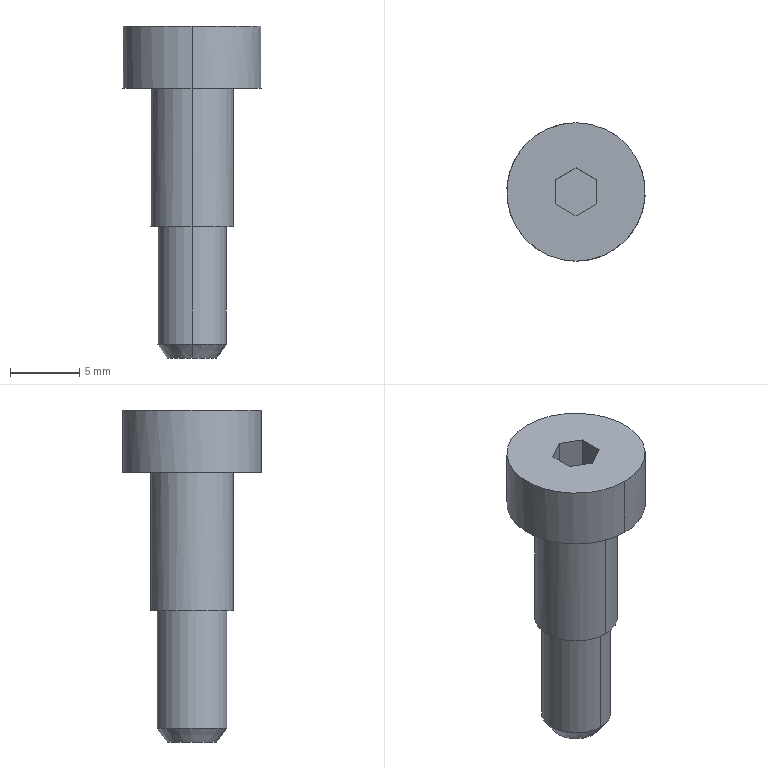Part | CATIA | 1 solid | 19 faces | box 10 x 10 x 24 mm | volume 794.336 mm3 | plane 11 | cylinder 6 | cone 2 | commonest cylinder face diameters 5 x2 6 x2 10 x2
STEP:
#1=CARTESIAN_POINT('',(0.,-2.5,-8.5));
#2=VERTEX_POINT('',#1);
#3=CARTESIAN_POINT('',(0.,-1.8,-9.5));
#4=VERTEX_POINT('',#3);
#5=CARTESIAN_POINT('',(0.,-286789.293,409565.487));
#6=DIRECTION('',(0.,-0.5736,0.8192));
#7=VECTOR('',#6,1.);
#8=LINE('',#5,#7);
#9=EDGE_CURVE('',#2,#4,#8,.F.);
#10=ORIENTED_EDGE('',*,*,#9,.F.);
#11=CARTESIAN_POINT('',(0.,2.5,-8.5));
#12=VERTEX_POINT('',#11);
#13=CARTESIAN_POINT('',(0.,0.,-8.5));
#14=DIRECTION('',(0.,0.,1.));
#15=AXIS2_PLACEMENT_3D('',#13,#14,$);
#16=CIRCLE('',#15,2.5);
#17=EDGE_CURVE('',#2,#12,#16,.F.);
#18=ORIENTED_EDGE('',*,*,#17,.T.);
#19=CARTESIAN_POINT('',(0.,1.8,-9.5));
#20=VERTEX_POINT('',#19);
#21=CARTESIAN_POINT('',(0.,286789.293,409565.487));
#22=DIRECTION('',(0.,0.5736,0.8192));
#23=VECTOR('',#22,1.);
#24=LINE('',#21,#23);
#25=EDGE_CURVE('',#20,#12,#24,.T.);
#26=ORIENTED_EDGE('',*,*,#25,.F.);
#27=CARTESIAN_POINT('',(0.,0.,-9.5));
#28=DIRECTION('',(0.,0.,1.));
#29=AXIS2_PLACEMENT_3D('',#27,#28,$);
#30=CIRCLE('',#29,1.8);
#31=EDGE_CURVE('',#4,#20,#30,.F.);
#32=ORIENTED_EDGE('',*,*,#31,.F.);
#33=EDGE_LOOP('',(#10,#18,#26,#32));
#34=FACE_OUTER_BOUND('',#33,.T.);
#35=CARTESIAN_POINT('',(0.,0.,-9.));
#36=DIRECTION('',(0.,0.,1.));
#37=DIRECTION('',(0.,1.,0.));
#38=AXIS2_PLACEMENT_3D('',#35,#36,#37);
#39=CONICAL_SURFACE('',#38,2.15,0.6109);
#40=ADVANCED_FACE('',(#34),#39,.T.);
#41=ORIENTED_EDGE('',*,*,#9,.T.);
#42=CARTESIAN_POINT('',(0.,0.,-9.5));
#43=DIRECTION('',(0.,0.,1.));
#44=AXIS2_PLACEMENT_3D('',#42,#43,$);
#45=CIRCLE('',#44,1.8);
#46=EDGE_CURVE('',#20,#4,#45,.F.);
#47=ORIENTED_EDGE('',*,*,#46,.F.);
#48=ORIENTED_EDGE('',*,*,#25,.T.);
#49=CARTESIAN_POINT('',(0.,0.,-8.5));
#50=DIRECTION('',(0.,0.,1.));
#51=AXIS2_PLACEMENT_3D('',#49,#50,$);
#52=CIRCLE('',#51,2.5);
#53=EDGE_CURVE('',#12,#2,#52,.F.);
#54=ORIENTED_EDGE('',*,*,#53,.T.);
#55=EDGE_LOOP('',(#41,#47,#48,#54));
#56=FACE_OUTER_BOUND('',#55,.T.);
#57=CARTESIAN_POINT('',(0.,0.,-9.));
#58=DIRECTION('',(0.,0.,1.));
#59=DIRECTION('',(0.,-1.,0.));
#60=AXIS2_PLACEMENT_3D('',#57,#58,#59);
#61=CONICAL_SURFACE('',#60,2.15,0.6109);
#62=ADVANCED_FACE('',(#56),#61,.T.);
#63=CARTESIAN_POINT('',(0.,-2.5,0.));
#64=VERTEX_POINT('',#63);
#65=CARTESIAN_POINT('',(0.,-2.5,-4.25));
#66=DIRECTION('',(0.,0.,1.));
#67=VECTOR('',#66,1.);
#68=LINE('',#65,#67);
#69=EDGE_CURVE('',#64,#2,#68,.F.);
#70=ORIENTED_EDGE('',*,*,#69,.F.);
#71=CARTESIAN_POINT('',(0.,2.5,0.));
#72=VERTEX_POINT('',#71);
#73=CARTESIAN_POINT('',(0.,0.,0.));
#74=DIRECTION('',(0.,0.,1.));
#75=AXIS2_PLACEMENT_3D('',#73,#74,$);
#76=CIRCLE('',#75,2.5);
#77=EDGE_CURVE('',#64,#72,#76,.F.);
#78=ORIENTED_EDGE('',*,*,#77,.T.);
#79=CARTESIAN_POINT('',(0.,2.5,-4.25));
#80=DIRECTION('',(0.,0.,1.));
#81=VECTOR('',#80,1.);
#82=LINE('',#79,#81);
#83=EDGE_CURVE('',#12,#72,#82,.T.);
#84=ORIENTED_EDGE('',*,*,#83,.F.);
#85=ORIENTED_EDGE('',*,*,#17,.F.);
#86=EDGE_LOOP('',(#70,#78,#84,#85));
#87=FACE_OUTER_BOUND('',#86,.T.);
#88=CARTESIAN_POINT('',(0.,0.,-4.25));
#89=DIRECTION('',(0.,0.,1.));
#90=DIRECTION('',(0.,1.,0.));
#91=AXIS2_PLACEMENT_3D('',#88,#89,#90);
#92=CYLINDRICAL_SURFACE('',#91,2.5);
#93=ADVANCED_FACE('',(#87),#92,.T.);
#94=ORIENTED_EDGE('',*,*,#31,.T.);
#95=ORIENTED_EDGE('',*,*,#46,.T.);
#96=EDGE_LOOP('',(#94,#95));
#97=FACE_OUTER_BOUND('',#96,.T.);
#98=CARTESIAN_POINT('',(0.,-0.8999,-9.5));
#99=DIRECTION('',(0.,0.,-1.));
#100=DIRECTION('',(0.,-1.,0.));
#101=AXIS2_PLACEMENT_3D('',#98,#99,#100);
#102=PLANE('',#101);
#103=ADVANCED_FACE('',(#97),#102,.T.);
#104=ORIENTED_EDGE('',*,*,#69,.T.);
#105=ORIENTED_EDGE('',*,*,#53,.F.);
#106=ORIENTED_EDGE('',*,*,#83,.T.);
#107=CARTESIAN_POINT('',(0.,0.,0.));
#108=DIRECTION('',(0.,0.,1.));
#109=AXIS2_PLACEMENT_3D('',#107,#108,$);
#110=CIRCLE('',#109,2.5);
#111=EDGE_CURVE('',#72,#64,#110,.F.);
#112=ORIENTED_EDGE('',*,*,#111,.T.);
#113=EDGE_LOOP('',(#104,#105,#106,#112));
#114=FACE_OUTER_BOUND('',#113,.T.);
#115=CARTESIAN_POINT('',(0.,0.,-4.25));
#116=DIRECTION('',(0.,0.,1.));
#117=DIRECTION('',(0.,-1.,0.));
#118=AXIS2_PLACEMENT_3D('',#115,#116,#117);
#119=CYLINDRICAL_SURFACE('',#118,2.5);
#120=ADVANCED_FACE('',(#114),#119,.T.);
#121=CARTESIAN_POINT('',(0.,-3.,0.));
#122=VERTEX_POINT('',#121);
#123=CARTESIAN_POINT('',(0.,3.,0.));
#124=VERTEX_POINT('',#123);
#125=CARTESIAN_POINT('',(0.,-3.,0.));
#126=CARTESIAN_POINT('',(-0.3394,-3.,0.));
#127=CARTESIAN_POINT('',(-0.6788,-2.952,0.));
#128=CARTESIAN_POINT('',(-1.009,-2.856,0.));
#129=CARTESIAN_POINT('',(-1.634,-2.573,0.));
#130=CARTESIAN_POINT('',(-2.155,-2.128,0.));
#131=CARTESIAN_POINT('',(-2.383,-1.87,0.));
#132=CARTESIAN_POINT('',(-2.758,-1.297,0.));
#133=CARTESIAN_POINT('',(-2.96,-0.6416,0.));
#134=CARTESIAN_POINT('',(-3.014,-0.3017,0.));
#135=CARTESIAN_POINT('',(-3.024,0.3838,0.));
#136=CARTESIAN_POINT('',(-2.843,1.045,0.));
#137=CARTESIAN_POINT('',(-2.706,1.361,0.));
#138=CARTESIAN_POINT('',(-2.347,1.945,0.));
#139=CARTESIAN_POINT('',(-1.84,2.406,0.));
#140=CARTESIAN_POINT('',(-1.555,2.599,0.));
#141=CARTESIAN_POINT('',(-1.077,2.833,0.));
#142=CARTESIAN_POINT('',(-0.5622,2.956,0.));
#143=CARTESIAN_POINT('',(-0.3758,2.985,0.));
#144=CARTESIAN_POINT('',(-0.1879,3.,0.));
#145=CARTESIAN_POINT('',(0.,3.,0.));
#146=B_SPLINE_CURVE_WITH_KNOTS('',5,(#125,#126,#127,#128,#129,#130,#131,#132,#133,#134,#135,#136,#137,#138,#139,#140,#141,#142,#143,#144,#145),.UNSPECIFIED.,.F.,.U.,(6,3,3,3,3,3,6),(0.,2.407,4.815,7.222,9.629,12.037,13.37),.UNSPECIFIED.);
#147=EDGE_CURVE('',#122,#124,#146,.T.);
#148=ORIENTED_EDGE('',*,*,#147,.T.);
#149=CARTESIAN_POINT('',(0.,3.,0.));
#150=CARTESIAN_POINT('',(0.3394,3.,0.));
#151=CARTESIAN_POINT('',(0.6788,2.952,0.));
#152=CARTESIAN_POINT('',(1.009,2.856,0.));
#153=CARTESIAN_POINT('',(1.634,2.573,0.));
#154=CARTESIAN_POINT('',(2.155,2.128,0.));
#155=CARTESIAN_POINT('',(2.383,1.87,0.));
#156=CARTESIAN_POINT('',(2.758,1.297,0.));
#157=CARTESIAN_POINT('',(2.96,0.6416,0.));
#158=CARTESIAN_POINT('',(3.014,0.3017,0.));
#159=CARTESIAN_POINT('',(3.024,-0.3838,0.));
#160=CARTESIAN_POINT('',(2.843,-1.045,0.));
#161=CARTESIAN_POINT('',(2.706,-1.361,0.));
#162=CARTESIAN_POINT('',(2.347,-1.945,0.));
#163=CARTESIAN_POINT('',(1.84,-2.406,0.));
#164=CARTESIAN_POINT('',(1.555,-2.599,0.));
#165=CARTESIAN_POINT('',(1.077,-2.833,0.));
#166=CARTESIAN_POINT('',(0.5622,-2.956,0.));
#167=CARTESIAN_POINT('',(0.3758,-2.985,0.));
#168=CARTESIAN_POINT('',(0.1879,-3.,0.));
#169=CARTESIAN_POINT('',(0.,-3.,0.));
#170=B_SPLINE_CURVE_WITH_KNOTS('',5,(#149,#150,#151,#152,#153,#154,#155,#156,#157,#158,#159,#160,#161,#162,#163,#164,#165,#166,#167,#168,#169),.UNSPECIFIED.,.F.,.U.,(6,3,3,3,3,3,6),(0.,2.407,4.815,7.222,9.629,12.037,13.37),.UNSPECIFIED.);
#171=EDGE_CURVE('',#124,#122,#170,.T.);
#172=ORIENTED_EDGE('',*,*,#171,.T.);
#173=EDGE_LOOP('',(#148,#172));
#174=FACE_OUTER_BOUND('',#173,.T.);
#175=ORIENTED_EDGE('',*,*,#77,.F.);
#176=ORIENTED_EDGE('',*,*,#111,.F.);
#177=EDGE_LOOP('',(#175,#176));
#178=FACE_BOUND('',#177,.T.);
#179=CARTESIAN_POINT('',(0.,-2.75,0.));
#180=DIRECTION('',(0.,0.,-1.));
#181=DIRECTION('',(0.,-1.,0.));
#182=AXIS2_PLACEMENT_3D('',#179,#180,#181);
#183=PLANE('',#182);
#184=ADVANCED_FACE('',(#174,#178),#183,.T.);
#185=CARTESIAN_POINT('',(0.,-3.,10.));
#186=VERTEX_POINT('',#185);
#187=CARTESIAN_POINT('',(0.,-3.,5.));
#188=DIRECTION('',(0.,0.,1.));
#189=VECTOR('',#188,1.);
#190=LINE('',#187,#189);
#191=EDGE_CURVE('',#186,#122,#190,.F.);
#192=ORIENTED_EDGE('',*,*,#191,.F.);
#193=CARTESIAN_POINT('',(0.,3.,10.));
#194=VERTEX_POINT('',#193);
#195=CARTESIAN_POINT('',(0.,0.,10.));
#196=DIRECTION('',(0.,0.,1.));
#197=AXIS2_PLACEMENT_3D('',#195,#196,$);
#198=CIRCLE('',#197,3.);
#199=EDGE_CURVE('',#186,#194,#198,.F.);
#200=ORIENTED_EDGE('',*,*,#199,.T.);
#201=CARTESIAN_POINT('',(0.,3.,5.));
#202=DIRECTION('',(0.,0.,1.));
#203=VECTOR('',#202,1.);
#204=LINE('',#201,#203);
#205=EDGE_CURVE('',#124,#194,#204,.T.);
#206=ORIENTED_EDGE('',*,*,#205,.F.);
#207=ORIENTED_EDGE('',*,*,#147,.F.);
#208=EDGE_LOOP('',(#192,#200,#206,#207));
#209=FACE_OUTER_BOUND('',#208,.T.);
#210=CARTESIAN_POINT('',(0.,0.,5.));
#211=DIRECTION('',(0.,0.,1.));
#212=DIRECTION('',(0.,1.,0.));
#213=AXIS2_PLACEMENT_3D('',#210,#211,#212);
#214=CYLINDRICAL_SURFACE('',#213,3.);
#215=ADVANCED_FACE('',(#209),#214,.T.);
#216=ORIENTED_EDGE('',*,*,#191,.T.);
#217=ORIENTED_EDGE('',*,*,#171,.F.);
#218=ORIENTED_EDGE('',*,*,#205,.T.);
#219=CARTESIAN_POINT('',(0.,0.,10.));
#220=DIRECTION('',(0.,0.,1.));
#221=AXIS2_PLACEMENT_3D('',#219,#220,$);
#222=CIRCLE('',#221,3.);
#223=EDGE_CURVE('',#194,#186,#222,.F.);
#224=ORIENTED_EDGE('',*,*,#223,.T.);
#225=EDGE_LOOP('',(#216,#217,#218,#224));
#226=FACE_OUTER_BOUND('',#225,.T.);
#227=CARTESIAN_POINT('',(0.,0.,5.));
#228=DIRECTION('',(0.,0.,1.));
#229=DIRECTION('',(0.,-1.,0.));
#230=AXIS2_PLACEMENT_3D('',#227,#228,#229);
#231=CYLINDRICAL_SURFACE('',#230,3.);
#232=ADVANCED_FACE('',(#226),#231,.T.);
#233=CARTESIAN_POINT('',(0.,-5.,10.));
#234=VERTEX_POINT('',#233);
#235=CARTESIAN_POINT('',(0.,5.,10.));
#236=VERTEX_POINT('',#235);
#237=CARTESIAN_POINT('',(0.,-5.,10.));
#238=CARTESIAN_POINT('',(-0.5477,-5.,10.));
#239=CARTESIAN_POINT('',(-1.095,-4.925,10.));
#240=CARTESIAN_POINT('',(-1.63,-4.775,10.));
#241=CARTESIAN_POINT('',(-2.643,-4.333,10.));
#242=CARTESIAN_POINT('',(-3.5,-3.634,10.));
#243=CARTESIAN_POINT('',(-3.878,-3.228,10.));
#244=CARTESIAN_POINT('',(-4.512,-2.323,10.));
#245=CARTESIAN_POINT('',(-4.88,-1.28,10.));
#246=CARTESIAN_POINT('',(-4.991,-0.7365,10.));
#247=CARTESIAN_POINT('',(-5.062,0.3669,10.));
#248=CARTESIAN_POINT('',(-4.833,1.449,10.));
#249=CARTESIAN_POINT('',(-4.645,1.97,10.));
#250=CARTESIAN_POINT('',(-4.13,2.949,10.));
#251=CARTESIAN_POINT('',(-3.372,3.753,10.));
#252=CARTESIAN_POINT('',(-2.939,4.101,10.));
#253=CARTESIAN_POINT('',(-2.116,4.593,10.));
#254=CARTESIAN_POINT('',(-1.204,4.878,10.));
#255=CARTESIAN_POINT('',(-0.806,4.959,10.));
#256=CARTESIAN_POINT('',(-0.403,5.,10.));
#257=CARTESIAN_POINT('',(0.,5.,10.));
#258=B_SPLINE_CURVE_WITH_KNOTS('',5,(#237,#238,#239,#240,#241,#242,#243,#244,#245,#246,#247,#248,#249,#250,#251,#252,#253,#254,#255,#256,#257),.UNSPECIFIED.,.F.,.U.,(6,3,3,3,3,3,6),(0.,3.884,7.768,11.653,15.537,19.421,22.279),.UNSPECIFIED.);
#259=EDGE_CURVE('',#234,#236,#258,.T.);
#260=ORIENTED_EDGE('',*,*,#259,.T.);
#261=CARTESIAN_POINT('',(0.,5.,10.));
#262=CARTESIAN_POINT('',(0.5477,5.,10.));
#263=CARTESIAN_POINT('',(1.095,4.925,10.));
#264=CARTESIAN_POINT('',(1.63,4.775,10.));
#265=CARTESIAN_POINT('',(2.643,4.333,10.));
#266=CARTESIAN_POINT('',(3.5,3.634,10.));
#267=CARTESIAN_POINT('',(3.878,3.228,10.));
#268=CARTESIAN_POINT('',(4.512,2.323,10.));
#269=CARTESIAN_POINT('',(4.88,1.28,10.));
#270=CARTESIAN_POINT('',(4.991,0.7365,10.));
#271=CARTESIAN_POINT('',(5.062,-0.3669,10.));
#272=CARTESIAN_POINT('',(4.833,-1.449,10.));
#273=CARTESIAN_POINT('',(4.645,-1.97,10.));
#274=CARTESIAN_POINT('',(4.13,-2.949,10.));
#275=CARTESIAN_POINT('',(3.372,-3.753,10.));
#276=CARTESIAN_POINT('',(2.939,-4.101,10.));
#277=CARTESIAN_POINT('',(2.116,-4.593,10.));
#278=CARTESIAN_POINT('',(1.204,-4.878,10.));
#279=CARTESIAN_POINT('',(0.806,-4.959,10.));
#280=CARTESIAN_POINT('',(0.403,-5.,10.));
#281=CARTESIAN_POINT('',(0.,-5.,10.));
#282=B_SPLINE_CURVE_WITH_KNOTS('',5,(#261,#262,#263,#264,#265,#266,#267,#268,#269,#270,#271,#272,#273,#274,#275,#276,#277,#278,#279,#280,#281),.UNSPECIFIED.,.F.,.U.,(6,3,3,3,3,3,6),(0.,3.884,7.768,11.653,15.537,19.421,22.279),.UNSPECIFIED.);
#283=EDGE_CURVE('',#236,#234,#282,.T.);
#284=ORIENTED_EDGE('',*,*,#283,.T.);
#285=EDGE_LOOP('',(#260,#284));
#286=FACE_OUTER_BOUND('',#285,.T.);
#287=ORIENTED_EDGE('',*,*,#199,.F.);
#288=ORIENTED_EDGE('',*,*,#223,.F.);
#289=EDGE_LOOP('',(#287,#288));
#290=FACE_BOUND('',#289,.T.);
#291=CARTESIAN_POINT('',(0.,-4.,10.));
#292=DIRECTION('',(0.,0.,-1.));
#293=DIRECTION('',(0.,-1.,0.));
#294=AXIS2_PLACEMENT_3D('',#291,#292,#293);
#295=PLANE('',#294);
#296=ADVANCED_FACE('',(#286,#290),#295,.T.);
#297=CARTESIAN_POINT('',(0.,-5.,14.5));
#298=VERTEX_POINT('',#297);
#299=CARTESIAN_POINT('',(0.,-5.,12.25));
#300=DIRECTION('',(0.,0.,1.));
#301=VECTOR('',#300,1.);
#302=LINE('',#299,#301);
#303=EDGE_CURVE('',#298,#234,#302,.F.);
#304=ORIENTED_EDGE('',*,*,#303,.F.);
#305=CARTESIAN_POINT('',(0.,5.,14.5));
#306=VERTEX_POINT('',#305);
#307=CARTESIAN_POINT('',(0.,0.,14.5));
#308=DIRECTION('',(0.,0.,1.));
#309=AXIS2_PLACEMENT_3D('',#307,#308,$);
#310=CIRCLE('',#309,5.);
#311=EDGE_CURVE('',#298,#306,#310,.F.);
#312=ORIENTED_EDGE('',*,*,#311,.T.);
#313=CARTESIAN_POINT('',(0.,5.,12.25));
#314=DIRECTION('',(0.,0.,1.));
#315=VECTOR('',#314,1.);
#316=LINE('',#313,#315);
#317=EDGE_CURVE('',#236,#306,#316,.T.);
#318=ORIENTED_EDGE('',*,*,#317,.F.);
#319=ORIENTED_EDGE('',*,*,#259,.F.);
#320=EDGE_LOOP('',(#304,#312,#318,#319));
#321=FACE_OUTER_BOUND('',#320,.T.);
#322=CARTESIAN_POINT('',(0.,0.,12.25));
#323=DIRECTION('',(0.,0.,1.));
#324=DIRECTION('',(0.,1.,0.));
#325=AXIS2_PLACEMENT_3D('',#322,#323,#324);
#326=CYLINDRICAL_SURFACE('',#325,5.);
#327=ADVANCED_FACE('',(#321),#326,.T.);
#328=ORIENTED_EDGE('',*,*,#303,.T.);
#329=ORIENTED_EDGE('',*,*,#283,.F.);
#330=ORIENTED_EDGE('',*,*,#317,.T.);
#331=CARTESIAN_POINT('',(0.,0.,14.5));
#332=DIRECTION('',(0.,0.,1.));
#333=AXIS2_PLACEMENT_3D('',#331,#332,$);
#334=CIRCLE('',#333,5.);
#335=EDGE_CURVE('',#306,#298,#334,.F.);
#336=ORIENTED_EDGE('',*,*,#335,.T.);
#337=EDGE_LOOP('',(#328,#329,#330,#336));
#338=FACE_OUTER_BOUND('',#337,.T.);
#339=CARTESIAN_POINT('',(0.,0.,12.25));
#340=DIRECTION('',(0.,0.,1.));
#341=DIRECTION('',(0.,-1.,0.));
#342=AXIS2_PLACEMENT_3D('',#339,#340,#341);
#343=CYLINDRICAL_SURFACE('',#342,5.);
#344=ADVANCED_FACE('',(#338),#343,.T.);
#345=ORIENTED_EDGE('',*,*,#311,.F.);
#346=ORIENTED_EDGE('',*,*,#335,.F.);
#347=EDGE_LOOP('',(#345,#346));
#348=FACE_OUTER_BOUND('',#347,.T.);
#349=CARTESIAN_POINT('',(-1.5,-0.866,14.5));
#350=VERTEX_POINT('',#349);
#351=CARTESIAN_POINT('',(-1.5,0.866,14.5));
#352=VERTEX_POINT('',#351);
#353=CARTESIAN_POINT('',(-1.5,-0.000000001,14.5));
#354=DIRECTION('',(0.,1.,0.));
#355=VECTOR('',#354,1.);
#356=LINE('',#353,#355);
#357=EDGE_CURVE('',#350,#352,#356,.T.);
#358=ORIENTED_EDGE('',*,*,#357,.T.);
#359=CARTESIAN_POINT('',(0.,1.732,14.5));
#360=VERTEX_POINT('',#359);
#361=CARTESIAN_POINT('',(-0.75,1.299,14.5));
#362=DIRECTION('',(0.866,0.5,0.));
#363=VECTOR('',#362,1.);
#364=LINE('',#361,#363);
#365=EDGE_CURVE('',#352,#360,#364,.T.);
#366=ORIENTED_EDGE('',*,*,#365,.T.);
#367=CARTESIAN_POINT('',(1.5,0.866,14.5));
#368=VERTEX_POINT('',#367);
#369=CARTESIAN_POINT('',(0.75,1.299,14.5));
#370=DIRECTION('',(0.866,-0.5,0.));
#371=VECTOR('',#370,1.);
#372=LINE('',#369,#371);
#373=EDGE_CURVE('',#360,#368,#372,.T.);
#374=ORIENTED_EDGE('',*,*,#373,.T.);
#375=CARTESIAN_POINT('',(1.5,-0.866,14.5));
#376=VERTEX_POINT('',#375);
#377=CARTESIAN_POINT('',(1.5,0.000000001,14.5));
#378=DIRECTION('',(0.,-1.,0.));
#379=VECTOR('',#378,1.);
#380=LINE('',#377,#379);
#381=EDGE_CURVE('',#368,#376,#380,.T.);
#382=ORIENTED_EDGE('',*,*,#381,.T.);
#383=CARTESIAN_POINT('',(0.,-1.732,14.5));
#384=VERTEX_POINT('',#383);
#385=CARTESIAN_POINT('',(0.75,-1.299,14.5));
#386=DIRECTION('',(-0.866,-0.5,0.));
#387=VECTOR('',#386,1.);
#388=LINE('',#385,#387);
#389=EDGE_CURVE('',#376,#384,#388,.T.);
#390=ORIENTED_EDGE('',*,*,#389,.T.);
#391=CARTESIAN_POINT('',(-0.75,-1.299,14.5));
#392=DIRECTION('',(-0.866,0.5,0.));
#393=VECTOR('',#392,1.);
#394=LINE('',#391,#393);
#395=EDGE_CURVE('',#384,#350,#394,.T.);
#396=ORIENTED_EDGE('',*,*,#395,.T.);
#397=EDGE_LOOP('',(#358,#366,#374,#382,#390,#396));
#398=FACE_BOUND('',#397,.T.);
#399=CARTESIAN_POINT('',(0.,-2.5,14.5));
#400=DIRECTION('',(0.,0.,1.));
#401=DIRECTION('',(0.,1.,0.));
#402=AXIS2_PLACEMENT_3D('',#399,#400,#401);
#403=PLANE('',#402);
#404=ADVANCED_FACE('',(#348,#398),#403,.T.);
#405=CARTESIAN_POINT('',(-1.5,0.866,11.5));
#406=VERTEX_POINT('',#405);
#407=CARTESIAN_POINT('',(-1.5,-0.866,11.5));
#408=VERTEX_POINT('',#407);
#409=CARTESIAN_POINT('',(-1.5,0.,11.5));
#410=DIRECTION('',(0.,-1.,0.));
#411=VECTOR('',#410,1.);
#412=LINE('',#409,#411);
#413=EDGE_CURVE('',#406,#408,#412,.T.);
#414=ORIENTED_EDGE('',*,*,#413,.F.);
#415=CARTESIAN_POINT('',(-1.5,0.866,13.));
#416=DIRECTION('',(0.,0.,-1.));
#417=VECTOR('',#416,1.);
#418=LINE('',#415,#417);
#419=EDGE_CURVE('',#352,#406,#418,.T.);
#420=ORIENTED_EDGE('',*,*,#419,.F.);
#421=ORIENTED_EDGE('',*,*,#357,.F.);
#422=CARTESIAN_POINT('',(-1.5,-0.866,13.));
#423=DIRECTION('',(0.,0.,-1.));
#424=VECTOR('',#423,1.);
#425=LINE('',#422,#424);
#426=EDGE_CURVE('',#350,#408,#425,.T.);
#427=ORIENTED_EDGE('',*,*,#426,.T.);
#428=EDGE_LOOP('',(#414,#420,#421,#427));
#429=FACE_OUTER_BOUND('',#428,.T.);
#430=CARTESIAN_POINT('',(-1.5,0.866,14.5));
#431=DIRECTION('',(-1.,0.,0.));
#432=DIRECTION('',(0.,1.,0.));
#433=AXIS2_PLACEMENT_3D('',#430,#431,#432);
#434=PLANE('',#433);
#435=ADVANCED_FACE('',(#429),#434,.F.);
#436=CARTESIAN_POINT('',(0.,1.732,11.5));
#437=VERTEX_POINT('',#436);
#438=CARTESIAN_POINT('',(-0.75,1.299,11.5));
#439=DIRECTION('',(-0.866,-0.5,0.));
#440=VECTOR('',#439,1.);
#441=LINE('',#438,#440);
#442=EDGE_CURVE('',#437,#406,#441,.T.);
#443=ORIENTED_EDGE('',*,*,#442,.F.);
#444=CARTESIAN_POINT('',(0.,1.732,13.));
#445=DIRECTION('',(0.,0.,-1.));
#446=VECTOR('',#445,1.);
#447=LINE('',#444,#446);
#448=EDGE_CURVE('',#360,#437,#447,.T.);
#449=ORIENTED_EDGE('',*,*,#448,.F.);
#450=ORIENTED_EDGE('',*,*,#365,.F.);
#451=ORIENTED_EDGE('',*,*,#419,.T.);
#452=EDGE_LOOP('',(#443,#449,#450,#451));
#453=FACE_OUTER_BOUND('',#452,.T.);
#454=CARTESIAN_POINT('',(0.,1.732,14.5));
#455=DIRECTION('',(-0.5,0.866,0.));
#456=DIRECTION('',(0.866,0.5,0.));
#457=AXIS2_PLACEMENT_3D('',#454,#455,#456);
#458=PLANE('',#457);
#459=ADVANCED_FACE('',(#453),#458,.F.);
#460=CARTESIAN_POINT('',(1.5,0.866,11.5));
#461=VERTEX_POINT('',#460);
#462=CARTESIAN_POINT('',(0.75,1.299,11.5));
#463=DIRECTION('',(-0.866,0.5,0.));
#464=VECTOR('',#463,1.);
#465=LINE('',#462,#464);
#466=EDGE_CURVE('',#461,#437,#465,.T.);
#467=ORIENTED_EDGE('',*,*,#466,.F.);
#468=CARTESIAN_POINT('',(1.5,0.866,13.));
#469=DIRECTION('',(0.,0.,-1.));
#470=VECTOR('',#469,1.);
#471=LINE('',#468,#470);
#472=EDGE_CURVE('',#368,#461,#471,.T.);
#473=ORIENTED_EDGE('',*,*,#472,.F.);
#474=ORIENTED_EDGE('',*,*,#373,.F.);
#475=ORIENTED_EDGE('',*,*,#448,.T.);
#476=EDGE_LOOP('',(#467,#473,#474,#475));
#477=FACE_OUTER_BOUND('',#476,.T.);
#478=CARTESIAN_POINT('',(1.5,0.866,14.5));
#479=DIRECTION('',(0.5,0.866,0.));
#480=DIRECTION('',(0.866,-0.5,0.));
#481=AXIS2_PLACEMENT_3D('',#478,#479,#480);
#482=PLANE('',#481);
#483=ADVANCED_FACE('',(#477),#482,.F.);
#484=CARTESIAN_POINT('',(1.5,-0.866,11.5));
#485=VERTEX_POINT('',#484);
#486=CARTESIAN_POINT('',(1.5,0.,11.5));
#487=DIRECTION('',(0.,1.,0.));
#488=VECTOR('',#487,1.);
#489=LINE('',#486,#488);
#490=EDGE_CURVE('',#485,#461,#489,.T.);
#491=ORIENTED_EDGE('',*,*,#490,.F.);
#492=CARTESIAN_POINT('',(1.5,-0.866,13.));
#493=DIRECTION('',(0.,0.,-1.));
#494=VECTOR('',#493,1.);
#495=LINE('',#492,#494);
#496=EDGE_CURVE('',#376,#485,#495,.T.);
#497=ORIENTED_EDGE('',*,*,#496,.F.);
#498=ORIENTED_EDGE('',*,*,#381,.F.);
#499=ORIENTED_EDGE('',*,*,#472,.T.);
#500=EDGE_LOOP('',(#491,#497,#498,#499));
#501=FACE_OUTER_BOUND('',#500,.T.);
#502=CARTESIAN_POINT('',(1.5,-0.866,14.5));
#503=DIRECTION('',(1.,0.,0.));
#504=DIRECTION('',(0.,-1.,0.));
#505=AXIS2_PLACEMENT_3D('',#502,#503,#504);
#506=PLANE('',#505);
#507=ADVANCED_FACE('',(#501),#506,.F.);
#508=CARTESIAN_POINT('',(0.,-1.732,11.5));
#509=VERTEX_POINT('',#508);
#510=CARTESIAN_POINT('',(0.75,-1.299,11.5));
#511=DIRECTION('',(0.866,0.5,0.));
#512=VECTOR('',#511,1.);
#513=LINE('',#510,#512);
#514=EDGE_CURVE('',#509,#485,#513,.T.);
#515=ORIENTED_EDGE('',*,*,#514,.F.);
#516=CARTESIAN_POINT('',(0.,-1.732,13.));
#517=DIRECTION('',(0.,0.,-1.));
#518=VECTOR('',#517,1.);
#519=LINE('',#516,#518);
#520=EDGE_CURVE('',#384,#509,#519,.T.);
#521=ORIENTED_EDGE('',*,*,#520,.F.);
#522=ORIENTED_EDGE('',*,*,#389,.F.);
#523=ORIENTED_EDGE('',*,*,#496,.T.);
#524=EDGE_LOOP('',(#515,#521,#522,#523));
#525=FACE_OUTER_BOUND('',#524,.T.);
#526=CARTESIAN_POINT('',(0.,-1.732,14.5));
#527=DIRECTION('',(0.5,-0.866,0.));
#528=DIRECTION('',(-0.866,-0.5,0.));
#529=AXIS2_PLACEMENT_3D('',#526,#527,#528);
#530=PLANE('',#529);
#531=ADVANCED_FACE('',(#525),#530,.F.);
#532=CARTESIAN_POINT('',(-0.75,-1.299,11.5));
#533=DIRECTION('',(0.866,-0.5,0.));
#534=VECTOR('',#533,1.);
#535=LINE('',#532,#534);
#536=EDGE_CURVE('',#408,#509,#535,.T.);
#537=ORIENTED_EDGE('',*,*,#536,.F.);
#538=ORIENTED_EDGE('',*,*,#426,.F.);
#539=ORIENTED_EDGE('',*,*,#395,.F.);
#540=ORIENTED_EDGE('',*,*,#520,.T.);
#541=EDGE_LOOP('',(#537,#538,#539,#540));
#542=FACE_OUTER_BOUND('',#541,.T.);
#543=CARTESIAN_POINT('',(-1.5,-0.866,14.5));
#544=DIRECTION('',(-0.5,-0.866,0.));
#545=DIRECTION('',(-0.866,0.5,0.));
#546=AXIS2_PLACEMENT_3D('',#543,#544,#545);
#547=PLANE('',#546);
#548=ADVANCED_FACE('',(#542),#547,.F.);
#549=ORIENTED_EDGE('',*,*,#413,.T.);
#550=ORIENTED_EDGE('',*,*,#536,.T.);
#551=ORIENTED_EDGE('',*,*,#514,.T.);
#552=ORIENTED_EDGE('',*,*,#490,.T.);
#553=ORIENTED_EDGE('',*,*,#466,.T.);
#554=ORIENTED_EDGE('',*,*,#442,.T.);
#555=EDGE_LOOP('',(#549,#550,#551,#552,#553,#554));
#556=FACE_OUTER_BOUND('',#555,.T.);
#557=CARTESIAN_POINT('',(0.,0.,11.5));
#558=DIRECTION('',(0.,0.,-1.));
#559=DIRECTION('',(1.,0.,0.));
#560=AXIS2_PLACEMENT_3D('',#557,#558,#559);
#561=PLANE('',#560);
#562=ADVANCED_FACE('',(#556),#561,.F.);
#563=CLOSED_SHELL('',(#40,#62,#93,#103,#120,#184,#215,#232,#296,#327,#344,#404,#435,#459,#483,#507,#531,#548,#562));
#564=MANIFOLD_SOLID_BREP('',#563);
#565=(LENGTH_UNIT()NAMED_UNIT(*)SI_UNIT(.MILLI.,.METRE.));
#566=UNCERTAINTY_MEASURE_WITH_UNIT(LENGTH_MEASURE(0.005),#565,'','');
#567=(NAMED_UNIT(*)PLANE_ANGLE_UNIT()SI_UNIT($,.RADIAN.));
#568=(NAMED_UNIT(*)SI_UNIT($,.STERADIAN.)SOLID_ANGLE_UNIT());
#569=(GEOMETRIC_REPRESENTATION_CONTEXT(3)GLOBAL_UNCERTAINTY_ASSIGNED_CONTEXT((#566))GLOBAL_UNIT_ASSIGNED_CONTEXT((#565,#567,#568))REPRESENTATION_CONTEXT('',''));
#570=ADVANCED_BREP_SHAPE_REPRESENTATION('',(#564),#569);